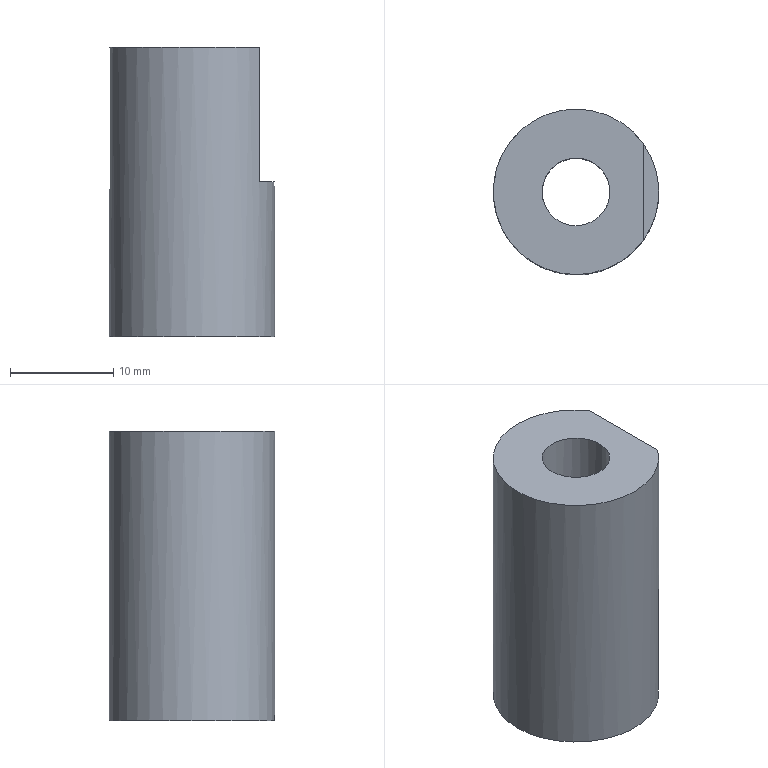Part | STEP file | lll_id146_x_t | 1 solid | 6 faces | box 16 x 16 x 28 mm | volume 4560 mm3 | plane 4 | cylinder 2 | commonest cylinder face diameters 6.56 x1 16 x1
STEP:
#1=CARTESIAN_POINT('',(797.273,-25.336,-13.));
#2=VERTEX_POINT('',#1);
#3=CARTESIAN_POINT('',(797.273,-34.664,-13.));
#4=VERTEX_POINT('',#3);
#5=CARTESIAN_POINT('',(797.273,-30.,-13.));
#6=DIRECTION('',(0.,-1.,0.));
#7=VECTOR('',#6,1.);
#8=LINE('',#5,#7);
#9=EDGE_CURVE('',#2,#4,#8,.T.);
#10=ORIENTED_EDGE('',*,*,#9,.F.);
#11=CARTESIAN_POINT('',(797.273,-25.336,0.));
#12=VERTEX_POINT('',#11);
#13=CARTESIAN_POINT('',(797.273,-25.336,-13.));
#14=DIRECTION('',(0.,0.,1.));
#15=VECTOR('',#14,1.);
#16=LINE('',#13,#15);
#17=EDGE_CURVE('',#2,#12,#16,.T.);
#18=ORIENTED_EDGE('',*,*,#17,.T.);
#19=CARTESIAN_POINT('',(797.273,-34.664,0.));
#20=VERTEX_POINT('',#19);
#21=CARTESIAN_POINT('',(797.273,-35.64,0.));
#22=DIRECTION('',(0.,1.,0.));
#23=VECTOR('',#22,1.);
#24=LINE('',#21,#23);
#25=EDGE_CURVE('',#20,#12,#24,.T.);
#26=ORIENTED_EDGE('',*,*,#25,.F.);
#27=CARTESIAN_POINT('',(797.273,-34.664,0.));
#28=DIRECTION('',(0.,0.,-1.));
#29=VECTOR('',#28,1.);
#30=LINE('',#27,#29);
#31=EDGE_CURVE('',#20,#4,#30,.T.);
#32=ORIENTED_EDGE('',*,*,#31,.T.);
#33=EDGE_LOOP('',(#10,#18,#26,#32));
#34=FACE_OUTER_BOUND('',#33,.T.);
#35=CARTESIAN_POINT('',(797.273,-35.64,-15.));
#36=DIRECTION('',(-1.,0.,0.));
#37=DIRECTION('',(0.,0.,-1.));
#38=AXIS2_PLACEMENT_3D('',#35,#36,#37);
#39=PLANE('',#38);
#40=ADVANCED_FACE('',(#34),#39,.F.);
#41=CARTESIAN_POINT('',(787.493,-30.,-28.));
#42=VERTEX_POINT('',#41);
#43=CARTESIAN_POINT('',(790.773,-30.,-28.));
#44=DIRECTION('',(0.,0.,-1.));
#45=DIRECTION('',(-1.,0.,0.));
#46=AXIS2_PLACEMENT_3D('',#43,#44,#45);
#47=CIRCLE('',#46,3.28);
#48=EDGE_CURVE('',#42,#42,#47,.T.);
#49=ORIENTED_EDGE('',*,*,#48,.F.);
#50=EDGE_LOOP('',(#49));
#51=FACE_BOUND('',#50,.T.);
#52=CARTESIAN_POINT('',(782.773,-30.,-28.));
#53=VERTEX_POINT('',#52);
#54=CARTESIAN_POINT('',(790.773,-30.,-28.));
#55=DIRECTION('',(0.,0.,1.));
#56=DIRECTION('',(-1.,0.,0.));
#57=AXIS2_PLACEMENT_3D('',#54,#55,#56);
#58=CIRCLE('',#57,8.);
#59=EDGE_CURVE('',#53,#53,#58,.T.);
#60=ORIENTED_EDGE('',*,*,#59,.F.);
#61=EDGE_LOOP('',(#60));
#62=FACE_BOUND('',#61,.T.);
#63=CARTESIAN_POINT('',(790.773,-30.,-28.));
#64=DIRECTION('',(0.,0.,-1.));
#65=DIRECTION('',(0.,1.,0.));
#66=AXIS2_PLACEMENT_3D('',#63,#64,#65);
#67=PLANE('',#66);
#68=ADVANCED_FACE('',(#51,#62),#67,.T.);
#69=CARTESIAN_POINT('',(790.773,-33.28,0.));
#70=VERTEX_POINT('',#69);
#71=CARTESIAN_POINT('',(790.773,-30.,0.));
#72=DIRECTION('',(0.,0.,1.));
#73=DIRECTION('',(0.,-1.,0.));
#74=AXIS2_PLACEMENT_3D('',#71,#72,#73);
#75=CIRCLE('',#74,3.28);
#76=EDGE_CURVE('',#70,#70,#75,.T.);
#77=ORIENTED_EDGE('',*,*,#76,.F.);
#78=EDGE_LOOP('',(#77));
#79=FACE_BOUND('',#78,.T.);
#80=ORIENTED_EDGE('',*,*,#25,.T.);
#81=CARTESIAN_POINT('',(790.773,-30.,0.));
#82=DIRECTION('',(0.,0.,-1.));
#83=DIRECTION('',(0.,-1.,0.));
#84=AXIS2_PLACEMENT_3D('',#81,#82,#83);
#85=CIRCLE('',#84,8.);
#86=EDGE_CURVE('',#20,#12,#85,.T.);
#87=ORIENTED_EDGE('',*,*,#86,.F.);
#88=EDGE_LOOP('',(#80,#87));
#89=FACE_BOUND('',#88,.T.);
#90=CARTESIAN_POINT('',(790.773,-30.,0.));
#91=DIRECTION('',(0.,0.,1.));
#92=DIRECTION('',(0.,-1.,0.));
#93=AXIS2_PLACEMENT_3D('',#90,#91,#92);
#94=PLANE('',#93);
#95=ADVANCED_FACE('',(#79,#89),#94,.T.);
#96=ORIENTED_EDGE('',*,*,#59,.T.);
#97=EDGE_LOOP('',(#96));
#98=FACE_BOUND('',#97,.T.);
#99=ORIENTED_EDGE('',*,*,#31,.F.);
#100=ORIENTED_EDGE('',*,*,#86,.T.);
#101=ORIENTED_EDGE('',*,*,#17,.F.);
#102=CARTESIAN_POINT('',(790.773,-30.,-13.));
#103=DIRECTION('',(0.,0.,-1.));
#104=DIRECTION('',(0.,-1.,0.));
#105=AXIS2_PLACEMENT_3D('',#102,#103,#104);
#106=CIRCLE('',#105,8.);
#107=EDGE_CURVE('',#2,#4,#106,.T.);
#108=ORIENTED_EDGE('',*,*,#107,.T.);
#109=EDGE_LOOP('',(#99,#100,#101,#108));
#110=FACE_BOUND('',#109,.T.);
#111=CARTESIAN_POINT('',(790.773,-30.,0.));
#112=DIRECTION('',(0.,0.,-1.));
#113=DIRECTION('',(0.,1.,0.));
#114=AXIS2_PLACEMENT_3D('',#111,#112,#113);
#115=CYLINDRICAL_SURFACE('',#114,8.);
#116=ADVANCED_FACE('',(#98,#110),#115,.T.);
#117=ORIENTED_EDGE('',*,*,#76,.T.);
#118=EDGE_LOOP('',(#117));
#119=FACE_BOUND('',#118,.T.);
#120=ORIENTED_EDGE('',*,*,#48,.T.);
#121=EDGE_LOOP('',(#120));
#122=FACE_BOUND('',#121,.T.);
#123=CARTESIAN_POINT('',(790.773,-30.,52.5));
#124=DIRECTION('',(0.,0.,-1.));
#125=DIRECTION('',(0.,1.,0.));
#126=AXIS2_PLACEMENT_3D('',#123,#124,#125);
#127=CYLINDRICAL_SURFACE('',#126,3.28);
#128=ADVANCED_FACE('',(#119,#122),#127,.F.);
#129=ORIENTED_EDGE('',*,*,#107,.F.);
#130=ORIENTED_EDGE('',*,*,#9,.T.);
#131=EDGE_LOOP('',(#129,#130));
#132=FACE_OUTER_BOUND('',#131,.T.);
#133=CARTESIAN_POINT('',(790.773,-30.,-13.));
#134=DIRECTION('',(0.,0.,1.));
#135=DIRECTION('',(0.,-1.,0.));
#136=AXIS2_PLACEMENT_3D('',#133,#134,#135);
#137=PLANE('',#136);
#138=ADVANCED_FACE('',(#132),#137,.T.);
#139=CLOSED_SHELL('',(#40,#68,#95,#116,#128,#138));
#140=MANIFOLD_SOLID_BREP('',#139);
#141=(LENGTH_UNIT()NAMED_UNIT(*)SI_UNIT(.MILLI.,.METRE.));
#142=UNCERTAINTY_MEASURE_WITH_UNIT(LENGTH_MEASURE(0.00002),#141,'','');
#143=(NAMED_UNIT(*)PLANE_ANGLE_UNIT()SI_UNIT($,.RADIAN.));
#144=PLANE_ANGLE_MEASURE_WITH_UNIT(PLANE_ANGLE_MEASURE(0.01745),#143);
#145=DIMENSIONAL_EXPONENTS(0.,0.,0.,0.,0.,0.,0.);
#146=(CONVERSION_BASED_UNIT('DEGREE',#144)NAMED_UNIT(#145)PLANE_ANGLE_UNIT());
#147=(NAMED_UNIT(*)SI_UNIT($,.STERADIAN.)SOLID_ANGLE_UNIT());
#148=(GEOMETRIC_REPRESENTATION_CONTEXT(3)GLOBAL_UNCERTAINTY_ASSIGNED_CONTEXT((#142))GLOBAL_UNIT_ASSIGNED_CONTEXT((#141,#146,#147))REPRESENTATION_CONTEXT('',''));
#149=ADVANCED_BREP_SHAPE_REPRESENTATION('',(#140),#148);